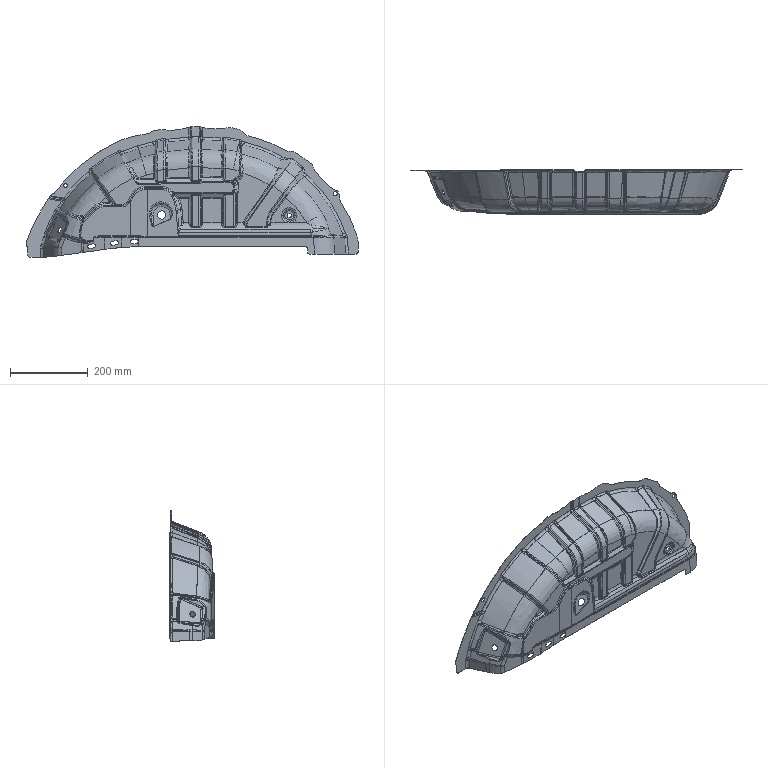Part | STEP file | FNA5401932 | 1 solid | 1328 faces | box 852.046 x 115.257 x 334.468 mm | volume 191833 mm3 | spline 1100 | cylinder 111 | plane 82 | sphere 24 | other 7 | torus 4 | commonest cylinder face diameters 10 x28 11.4 x18 16 x9 17.4 x9 8.6 x6 30 x6